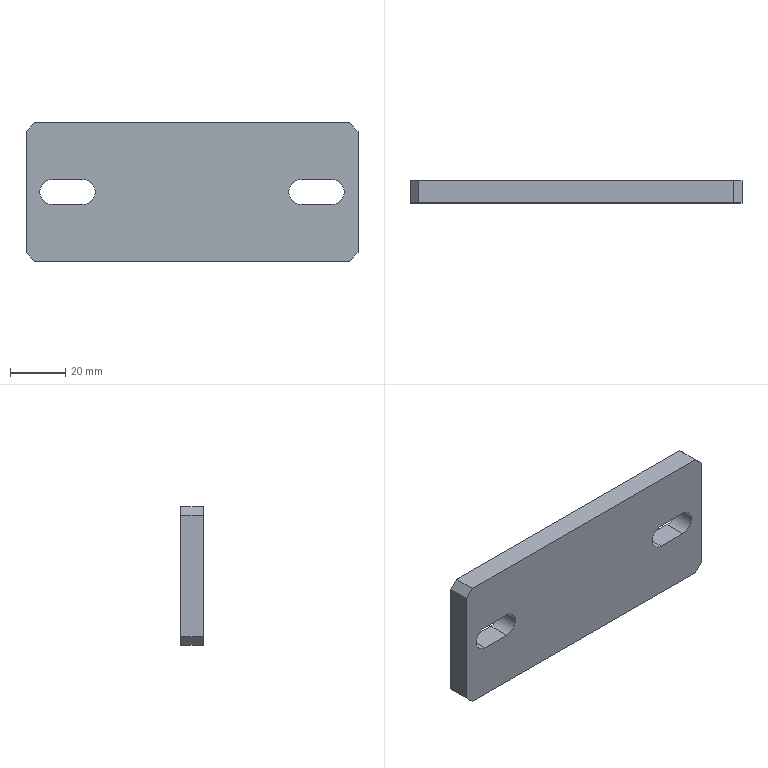Part | STEP file | PN_0013 304 stair handrail mounting plate 120X50X8_Default<As Machined> | 1 solid | 18 faces | box 120 x 8 x 50 mm | volume 45254 mm3 | plane 14 | cylinder 4 | commonest cylinder face diameters 9 x4
STEP:
#1=CARTESIAN_POINT('',(0.,0.,0.));
#2=DIRECTION('',(0.,0.,1.));
#3=DIRECTION('',(1.,0.,0.));
#4=AXIS2_PLACEMENT_3D('',#1,#2,#3);
#5=CARTESIAN_POINT('',(-50.5,0.,4.5));
#6=VERTEX_POINT('',#5);
#7=CARTESIAN_POINT('',(-39.5,0.,4.5));
#8=VERTEX_POINT('',#7);
#9=CARTESIAN_POINT('',(-50.5,0.,4.5));
#10=DIRECTION('',(1.,0.,0.));
#11=VECTOR('',#10,1.);
#12=LINE('',#9,#11);
#13=CARTESIAN_POINT('',(0.,0.,0.));
#14=DIRECTION('',(0.,-1.,0.));
#15=DIRECTION('',(0.,0.,-1.));
#16=AXIS2_PLACEMENT_3D('',#13,#14,#15);
#17=PLANE('',#16);
#18=CARTESIAN_POINT('',(-4.5,-50.5));
#19=DIRECTION('',(0.,1.));
#20=VECTOR('',#19,1.);
#21=LINE('',#18,#20);
#22=(GEOMETRIC_REPRESENTATION_CONTEXT(2)PARAMETRIC_REPRESENTATION_CONTEXT()REPRESENTATION_CONTEXT('',''));
#23=DEFINITIONAL_REPRESENTATION('',(#21),#22);
#24=PCURVE('',#17,#23);
#25=CARTESIAN_POINT('',(-50.5,8.,4.5));
#26=DIRECTION('',(0.,0.,1.));
#27=DIRECTION('',(1.,0.,0.));
#28=AXIS2_PLACEMENT_3D('',#25,#26,#27);
#29=PLANE('',#28);
#30=CARTESIAN_POINT('',(0.,-8.));
#31=DIRECTION('',(1.,0.));
#32=VECTOR('',#31,1.);
#33=LINE('',#30,#32);
#34=(GEOMETRIC_REPRESENTATION_CONTEXT(2)PARAMETRIC_REPRESENTATION_CONTEXT()REPRESENTATION_CONTEXT('',''));
#35=DEFINITIONAL_REPRESENTATION('',(#33),#34);
#36=PCURVE('',#29,#35);
#37=SURFACE_CURVE('',#12,(#24,#36),.PCURVE_S1.);
#38=EDGE_CURVE('',#6,#8,#37,.T.);
#39=ORIENTED_EDGE('',*,*,#38,.T.);
#40=CARTESIAN_POINT('',(-39.5,0.,-4.5));
#41=VERTEX_POINT('',#40);
#42=CARTESIAN_POINT('',(-39.5,0.,0.));
#43=DIRECTION('',(0.,1.,0.));
#44=DIRECTION('',(0.,0.,1.));
#45=AXIS2_PLACEMENT_3D('',#42,#43,#44);
#46=CIRCLE('',#45,4.5);
#47=CARTESIAN_POINT('',(-4.5,-39.5));
#48=CARTESIAN_POINT('',(-4.5,-31.706));
#49=CARTESIAN_POINT('',(2.25,-35.603));
#50=CARTESIAN_POINT('',(9.,-39.5));
#51=CARTESIAN_POINT('',(2.25,-43.397));
#52=CARTESIAN_POINT('',(-4.5,-47.294));
#53=CARTESIAN_POINT('',(-4.5,-39.5));
#54=(BOUNDED_CURVE()B_SPLINE_CURVE(2,(#47,#48,#49,#50,#51,#52,#53),.UNSPECIFIED.,.T.,.F.)B_SPLINE_CURVE_WITH_KNOTS((1,2,2,2,2,1),(-2.094,0.,2.094,4.189,6.283,8.378),.UNSPECIFIED.)CURVE()GEOMETRIC_REPRESENTATION_ITEM()RATIONAL_B_SPLINE_CURVE((1.,0.5,1.,0.5,1.,0.5,1.))REPRESENTATION_ITEM(''));
#55=(GEOMETRIC_REPRESENTATION_CONTEXT(2)PARAMETRIC_REPRESENTATION_CONTEXT()REPRESENTATION_CONTEXT('',''));
#56=DEFINITIONAL_REPRESENTATION('',(#54),#55);
#57=PCURVE('',#17,#56);
#58=CARTESIAN_POINT('',(-39.5,8.,0.));
#59=DIRECTION('',(0.,1.,0.));
#60=DIRECTION('',(0.,0.,1.));
#61=AXIS2_PLACEMENT_3D('',#58,#59,#60);
#62=CYLINDRICAL_SURFACE('',#61,4.5);
#63=CARTESIAN_POINT('',(0.,-8.));
#64=DIRECTION('',(1.,0.));
#65=VECTOR('',#64,1.);
#66=LINE('',#63,#65);
#67=(GEOMETRIC_REPRESENTATION_CONTEXT(2)PARAMETRIC_REPRESENTATION_CONTEXT()REPRESENTATION_CONTEXT('',''));
#68=DEFINITIONAL_REPRESENTATION('',(#66),#67);
#69=PCURVE('',#62,#68);
#70=SURFACE_CURVE('',#46,(#57,#69),.PCURVE_S1.);
#71=EDGE_CURVE('',#8,#41,#70,.T.);
#72=ORIENTED_EDGE('',*,*,#71,.T.);
#73=CARTESIAN_POINT('',(-50.5,0.,-4.5));
#74=VERTEX_POINT('',#73);
#75=CARTESIAN_POINT('',(-50.5,0.,-4.5));
#76=DIRECTION('',(1.,0.,0.));
#77=VECTOR('',#76,1.);
#78=LINE('',#75,#77);
#79=CARTESIAN_POINT('',(4.5,-50.5));
#80=DIRECTION('',(0.,1.));
#81=VECTOR('',#80,1.);
#82=LINE('',#79,#81);
#83=(GEOMETRIC_REPRESENTATION_CONTEXT(2)PARAMETRIC_REPRESENTATION_CONTEXT()REPRESENTATION_CONTEXT('',''));
#84=DEFINITIONAL_REPRESENTATION('',(#82),#83);
#85=PCURVE('',#17,#84);
#86=CARTESIAN_POINT('',(-50.5,8.,-4.5));
#87=DIRECTION('',(0.,0.,-1.));
#88=DIRECTION('',(-1.,0.,0.));
#89=AXIS2_PLACEMENT_3D('',#86,#87,#88);
#90=PLANE('',#89);
#91=CARTESIAN_POINT('',(0.,-8.));
#92=DIRECTION('',(-1.,0.));
#93=VECTOR('',#92,1.);
#94=LINE('',#91,#93);
#95=(GEOMETRIC_REPRESENTATION_CONTEXT(2)PARAMETRIC_REPRESENTATION_CONTEXT()REPRESENTATION_CONTEXT('',''));
#96=DEFINITIONAL_REPRESENTATION('',(#94),#95);
#97=PCURVE('',#90,#96);
#98=SURFACE_CURVE('',#78,(#85,#97),.PCURVE_S1.);
#99=EDGE_CURVE('',#74,#41,#98,.T.);
#100=ORIENTED_EDGE('',*,*,#99,.F.);
#101=CARTESIAN_POINT('',(-50.5,0.,0.));
#102=DIRECTION('',(0.,1.,0.));
#103=DIRECTION('',(0.,0.,1.));
#104=AXIS2_PLACEMENT_3D('',#101,#102,#103);
#105=CIRCLE('',#104,4.5);
#106=CARTESIAN_POINT('',(-4.5,-50.5));
#107=CARTESIAN_POINT('',(-4.5,-42.706));
#108=CARTESIAN_POINT('',(2.25,-46.603));
#109=CARTESIAN_POINT('',(9.,-50.5));
#110=CARTESIAN_POINT('',(2.25,-54.397));
#111=CARTESIAN_POINT('',(-4.5,-58.294));
#112=CARTESIAN_POINT('',(-4.5,-50.5));
#113=(BOUNDED_CURVE()B_SPLINE_CURVE(2,(#106,#107,#108,#109,#110,#111,#112),.UNSPECIFIED.,.T.,.F.)B_SPLINE_CURVE_WITH_KNOTS((1,2,2,2,2,1),(-2.094,0.,2.094,4.189,6.283,8.378),.UNSPECIFIED.)CURVE()GEOMETRIC_REPRESENTATION_ITEM()RATIONAL_B_SPLINE_CURVE((1.,0.5,1.,0.5,1.,0.5,1.))REPRESENTATION_ITEM(''));
#114=(GEOMETRIC_REPRESENTATION_CONTEXT(2)PARAMETRIC_REPRESENTATION_CONTEXT()REPRESENTATION_CONTEXT('',''));
#115=DEFINITIONAL_REPRESENTATION('',(#113),#114);
#116=PCURVE('',#17,#115);
#117=CARTESIAN_POINT('',(-50.5,8.,0.));
#118=DIRECTION('',(0.,1.,0.));
#119=DIRECTION('',(0.,0.,1.));
#120=AXIS2_PLACEMENT_3D('',#117,#118,#119);
#121=CYLINDRICAL_SURFACE('',#120,4.5);
#122=CARTESIAN_POINT('',(0.,-8.));
#123=DIRECTION('',(1.,0.));
#124=VECTOR('',#123,1.);
#125=LINE('',#122,#124);
#126=(GEOMETRIC_REPRESENTATION_CONTEXT(2)PARAMETRIC_REPRESENTATION_CONTEXT()REPRESENTATION_CONTEXT('',''));
#127=DEFINITIONAL_REPRESENTATION('',(#125),#126);
#128=PCURVE('',#121,#127);
#129=SURFACE_CURVE('',#105,(#116,#128),.PCURVE_S1.);
#130=EDGE_CURVE('',#74,#6,#129,.T.);
#131=ORIENTED_EDGE('',*,*,#130,.T.);
#132=EDGE_LOOP('',(#39,#72,#100,#131));
#133=FACE_BOUND('',#132,.T.);
#134=CARTESIAN_POINT('',(57.,0.,-25.));
#135=VERTEX_POINT('',#134);
#136=CARTESIAN_POINT('',(-57.,0.,-25.));
#137=VERTEX_POINT('',#136);
#138=CARTESIAN_POINT('',(-60.,0.,-25.));
#139=DIRECTION('',(-1.,0.,0.));
#140=VECTOR('',#139,1.);
#141=LINE('',#138,#140);
#142=CARTESIAN_POINT('',(25.,-60.));
#143=DIRECTION('',(0.,-1.));
#144=VECTOR('',#143,1.);
#145=LINE('',#142,#144);
#146=(GEOMETRIC_REPRESENTATION_CONTEXT(2)PARAMETRIC_REPRESENTATION_CONTEXT()REPRESENTATION_CONTEXT('',''));
#147=DEFINITIONAL_REPRESENTATION('',(#145),#146);
#148=PCURVE('',#17,#147);
#149=CARTESIAN_POINT('',(-60.,8.,-25.));
#150=DIRECTION('',(0.,0.,1.));
#151=DIRECTION('',(1.,0.,0.));
#152=AXIS2_PLACEMENT_3D('',#149,#150,#151);
#153=PLANE('',#152);
#154=CARTESIAN_POINT('',(0.,-8.));
#155=DIRECTION('',(-1.,0.));
#156=VECTOR('',#155,1.);
#157=LINE('',#154,#156);
#158=(GEOMETRIC_REPRESENTATION_CONTEXT(2)PARAMETRIC_REPRESENTATION_CONTEXT()REPRESENTATION_CONTEXT('',''));
#159=DEFINITIONAL_REPRESENTATION('',(#157),#158);
#160=PCURVE('',#153,#159);
#161=SURFACE_CURVE('',#141,(#148,#160),.PCURVE_S1.);
#162=EDGE_CURVE('',#135,#137,#161,.T.);
#163=ORIENTED_EDGE('',*,*,#162,.F.);
#164=CARTESIAN_POINT('',(60.,0.,-22.));
#165=VERTEX_POINT('',#164);
#166=CARTESIAN_POINT('',(41.,0.,-41.));
#167=DIRECTION('',(0.7071,0.,0.7071));
#168=VECTOR('',#167,1.);
#169=LINE('',#166,#168);
#170=CARTESIAN_POINT('',(41.,41.));
#171=DIRECTION('',(-0.7071,0.7071));
#172=VECTOR('',#171,1.);
#173=LINE('',#170,#172);
#174=(GEOMETRIC_REPRESENTATION_CONTEXT(2)PARAMETRIC_REPRESENTATION_CONTEXT()REPRESENTATION_CONTEXT('',''));
#175=DEFINITIONAL_REPRESENTATION('',(#173),#174);
#176=PCURVE('',#17,#175);
#177=CARTESIAN_POINT('',(57.,8.,-25.));
#178=DIRECTION('',(-0.7071,0.,0.7071));
#179=DIRECTION('',(0.,-1.,0.));
#180=AXIS2_PLACEMENT_3D('',#177,#178,#179);
#181=PLANE('',#180);
#182=CARTESIAN_POINT('',(8.,-22.627));
#183=DIRECTION('',(0.,1.));
#184=VECTOR('',#183,1.);
#185=LINE('',#182,#184);
#186=(GEOMETRIC_REPRESENTATION_CONTEXT(2)PARAMETRIC_REPRESENTATION_CONTEXT()REPRESENTATION_CONTEXT('',''));
#187=DEFINITIONAL_REPRESENTATION('',(#185),#186);
#188=PCURVE('',#181,#187);
#189=SURFACE_CURVE('',#169,(#176,#188),.PCURVE_S1.);
#190=EDGE_CURVE('',#135,#165,#189,.T.);
#191=ORIENTED_EDGE('',*,*,#190,.T.);
#192=CARTESIAN_POINT('',(60.,0.,22.));
#193=VERTEX_POINT('',#192);
#194=CARTESIAN_POINT('',(60.,0.,25.));
#195=DIRECTION('',(0.,0.,-1.));
#196=VECTOR('',#195,1.);
#197=LINE('',#194,#196);
#198=CARTESIAN_POINT('',(-25.,60.));
#199=DIRECTION('',(1.,0.));
#200=VECTOR('',#199,1.);
#201=LINE('',#198,#200);
#202=(GEOMETRIC_REPRESENTATION_CONTEXT(2)PARAMETRIC_REPRESENTATION_CONTEXT()REPRESENTATION_CONTEXT('',''));
#203=DEFINITIONAL_REPRESENTATION('',(#201),#202);
#204=PCURVE('',#17,#203);
#205=CARTESIAN_POINT('',(60.,8.,25.));
#206=DIRECTION('',(-1.,0.,0.));
#207=DIRECTION('',(0.,0.,1.));
#208=AXIS2_PLACEMENT_3D('',#205,#206,#207);
#209=PLANE('',#208);
#210=CARTESIAN_POINT('',(0.,-8.));
#211=DIRECTION('',(-1.,0.));
#212=VECTOR('',#211,1.);
#213=LINE('',#210,#212);
#214=(GEOMETRIC_REPRESENTATION_CONTEXT(2)PARAMETRIC_REPRESENTATION_CONTEXT()REPRESENTATION_CONTEXT('',''));
#215=DEFINITIONAL_REPRESENTATION('',(#213),#214);
#216=PCURVE('',#209,#215);
#217=SURFACE_CURVE('',#197,(#204,#216),.PCURVE_S1.);
#218=EDGE_CURVE('',#193,#165,#217,.T.);
#219=ORIENTED_EDGE('',*,*,#218,.F.);
#220=CARTESIAN_POINT('',(57.,0.,25.));
#221=VERTEX_POINT('',#220);
#222=CARTESIAN_POINT('',(41.,0.,41.));
#223=DIRECTION('',(-0.7071,0.,0.7071));
#224=VECTOR('',#223,1.);
#225=LINE('',#222,#224);
#226=CARTESIAN_POINT('',(-41.,41.));
#227=DIRECTION('',(-0.7071,-0.7071));
#228=VECTOR('',#227,1.);
#229=LINE('',#226,#228);
#230=(GEOMETRIC_REPRESENTATION_CONTEXT(2)PARAMETRIC_REPRESENTATION_CONTEXT()REPRESENTATION_CONTEXT('',''));
#231=DEFINITIONAL_REPRESENTATION('',(#229),#230);
#232=PCURVE('',#17,#231);
#233=CARTESIAN_POINT('',(60.,8.,22.));
#234=DIRECTION('',(-0.7071,0.,-0.7071));
#235=DIRECTION('',(0.,-1.,0.));
#236=AXIS2_PLACEMENT_3D('',#233,#234,#235);
#237=PLANE('',#236);
#238=CARTESIAN_POINT('',(8.,26.87));
#239=DIRECTION('',(0.,1.));
#240=VECTOR('',#239,1.);
#241=LINE('',#238,#240);
#242=(GEOMETRIC_REPRESENTATION_CONTEXT(2)PARAMETRIC_REPRESENTATION_CONTEXT()REPRESENTATION_CONTEXT('',''));
#243=DEFINITIONAL_REPRESENTATION('',(#241),#242);
#244=PCURVE('',#237,#243);
#245=SURFACE_CURVE('',#225,(#232,#244),.PCURVE_S1.);
#246=EDGE_CURVE('',#193,#221,#245,.T.);
#247=ORIENTED_EDGE('',*,*,#246,.T.);
#248=CARTESIAN_POINT('',(-57.,0.,25.));
#249=VERTEX_POINT('',#248);
#250=CARTESIAN_POINT('',(-60.,0.,25.));
#251=DIRECTION('',(1.,0.,0.));
#252=VECTOR('',#251,1.);
#253=LINE('',#250,#252);
#254=CARTESIAN_POINT('',(-25.,-60.));
#255=DIRECTION('',(0.,1.));
#256=VECTOR('',#255,1.);
#257=LINE('',#254,#256);
#258=(GEOMETRIC_REPRESENTATION_CONTEXT(2)PARAMETRIC_REPRESENTATION_CONTEXT()REPRESENTATION_CONTEXT('',''));
#259=DEFINITIONAL_REPRESENTATION('',(#257),#258);
#260=PCURVE('',#17,#259);
#261=CARTESIAN_POINT('',(-60.,8.,25.));
#262=DIRECTION('',(0.,0.,-1.));
#263=DIRECTION('',(-1.,0.,0.));
#264=AXIS2_PLACEMENT_3D('',#261,#262,#263);
#265=PLANE('',#264);
#266=CARTESIAN_POINT('',(0.,-8.));
#267=DIRECTION('',(-1.,0.));
#268=VECTOR('',#267,1.);
#269=LINE('',#266,#268);
#270=(GEOMETRIC_REPRESENTATION_CONTEXT(2)PARAMETRIC_REPRESENTATION_CONTEXT()REPRESENTATION_CONTEXT('',''));
#271=DEFINITIONAL_REPRESENTATION('',(#269),#270);
#272=PCURVE('',#265,#271);
#273=SURFACE_CURVE('',#253,(#260,#272),.PCURVE_S1.);
#274=EDGE_CURVE('',#249,#221,#273,.T.);
#275=ORIENTED_EDGE('',*,*,#274,.F.);
#276=CARTESIAN_POINT('',(-60.,0.,22.));
#277=VERTEX_POINT('',#276);
#278=CARTESIAN_POINT('',(-41.,0.,41.));
#279=DIRECTION('',(-0.7071,0.,-0.7071));
#280=VECTOR('',#279,1.);
#281=LINE('',#278,#280);
#282=CARTESIAN_POINT('',(-41.,-41.));
#283=DIRECTION('',(0.7071,-0.7071));
#284=VECTOR('',#283,1.);
#285=LINE('',#282,#284);
#286=(GEOMETRIC_REPRESENTATION_CONTEXT(2)PARAMETRIC_REPRESENTATION_CONTEXT()REPRESENTATION_CONTEXT('',''));
#287=DEFINITIONAL_REPRESENTATION('',(#285),#286);
#288=PCURVE('',#17,#287);
#289=CARTESIAN_POINT('',(-57.,8.,25.));
#290=DIRECTION('',(0.7071,0.,-0.7071));
#291=DIRECTION('',(0.,-1.,0.));
#292=AXIS2_PLACEMENT_3D('',#289,#290,#291);
#293=PLANE('',#292);
#294=CARTESIAN_POINT('',(8.,-22.627));
#295=DIRECTION('',(0.,1.));
#296=VECTOR('',#295,1.);
#297=LINE('',#294,#296);
#298=(GEOMETRIC_REPRESENTATION_CONTEXT(2)PARAMETRIC_REPRESENTATION_CONTEXT()REPRESENTATION_CONTEXT('',''));
#299=DEFINITIONAL_REPRESENTATION('',(#297),#298);
#300=PCURVE('',#293,#299);
#301=SURFACE_CURVE('',#281,(#288,#300),.PCURVE_S1.);
#302=EDGE_CURVE('',#249,#277,#301,.T.);
#303=ORIENTED_EDGE('',*,*,#302,.T.);
#304=CARTESIAN_POINT('',(-60.,0.,-22.));
#305=VERTEX_POINT('',#304);
#306=CARTESIAN_POINT('',(-60.,0.,25.));
#307=DIRECTION('',(0.,0.,1.));
#308=VECTOR('',#307,1.);
#309=LINE('',#306,#308);
#310=CARTESIAN_POINT('',(-25.,-60.));
#311=DIRECTION('',(-1.,0.));
#312=VECTOR('',#311,1.);
#313=LINE('',#310,#312);
#314=(GEOMETRIC_REPRESENTATION_CONTEXT(2)PARAMETRIC_REPRESENTATION_CONTEXT()REPRESENTATION_CONTEXT('',''));
#315=DEFINITIONAL_REPRESENTATION('',(#313),#314);
#316=PCURVE('',#17,#315);
#317=CARTESIAN_POINT('',(-60.,8.,25.));
#318=DIRECTION('',(1.,0.,0.));
#319=DIRECTION('',(0.,0.,-1.));
#320=AXIS2_PLACEMENT_3D('',#317,#318,#319);
#321=PLANE('',#320);
#322=CARTESIAN_POINT('',(0.,-8.));
#323=DIRECTION('',(-1.,0.));
#324=VECTOR('',#323,1.);
#325=LINE('',#322,#324);
#326=(GEOMETRIC_REPRESENTATION_CONTEXT(2)PARAMETRIC_REPRESENTATION_CONTEXT()REPRESENTATION_CONTEXT('',''));
#327=DEFINITIONAL_REPRESENTATION('',(#325),#326);
#328=PCURVE('',#321,#327);
#329=SURFACE_CURVE('',#309,(#316,#328),.PCURVE_S1.);
#330=EDGE_CURVE('',#305,#277,#329,.T.);
#331=ORIENTED_EDGE('',*,*,#330,.F.);
#332=CARTESIAN_POINT('',(-41.,0.,-41.));
#333=DIRECTION('',(0.7071,0.,-0.7071));
#334=VECTOR('',#333,1.);
#335=LINE('',#332,#334);
#336=CARTESIAN_POINT('',(41.,-41.));
#337=DIRECTION('',(0.7071,0.7071));
#338=VECTOR('',#337,1.);
#339=LINE('',#336,#338);
#340=(GEOMETRIC_REPRESENTATION_CONTEXT(2)PARAMETRIC_REPRESENTATION_CONTEXT()REPRESENTATION_CONTEXT('',''));
#341=DEFINITIONAL_REPRESENTATION('',(#339),#340);
#342=PCURVE('',#17,#341);
#343=CARTESIAN_POINT('',(-60.,8.,-22.));
#344=DIRECTION('',(0.7071,0.,0.7071));
#345=DIRECTION('',(0.,-1.,0.));
#346=AXIS2_PLACEMENT_3D('',#343,#344,#345);
#347=PLANE('',#346);
#348=CARTESIAN_POINT('',(8.,26.87));
#349=DIRECTION('',(0.,1.));
#350=VECTOR('',#349,1.);
#351=LINE('',#348,#350);
#352=(GEOMETRIC_REPRESENTATION_CONTEXT(2)PARAMETRIC_REPRESENTATION_CONTEXT()REPRESENTATION_CONTEXT('',''));
#353=DEFINITIONAL_REPRESENTATION('',(#351),#352);
#354=PCURVE('',#347,#353);
#355=SURFACE_CURVE('',#335,(#342,#354),.PCURVE_S1.);
#356=EDGE_CURVE('',#305,#137,#355,.T.);
#357=ORIENTED_EDGE('',*,*,#356,.T.);
#358=EDGE_LOOP('',(#163,#191,#219,#247,#275,#303,#331,#357));
#359=FACE_BOUND('',#358,.T.);
#360=CARTESIAN_POINT('',(39.5,0.,-4.5));
#361=VERTEX_POINT('',#360);
#362=CARTESIAN_POINT('',(39.5,0.,4.5));
#363=VERTEX_POINT('',#362);
#364=CARTESIAN_POINT('',(39.5,0.,0.));
#365=DIRECTION('',(0.,1.,0.));
#366=DIRECTION('',(0.,0.,1.));
#367=AXIS2_PLACEMENT_3D('',#364,#365,#366);
#368=CIRCLE('',#367,4.5);
#369=CARTESIAN_POINT('',(-4.5,39.5));
#370=CARTESIAN_POINT('',(-4.5,47.294));
#371=CARTESIAN_POINT('',(2.25,43.397));
#372=CARTESIAN_POINT('',(9.,39.5));
#373=CARTESIAN_POINT('',(2.25,35.603));
#374=CARTESIAN_POINT('',(-4.5,31.706));
#375=CARTESIAN_POINT('',(-4.5,39.5));
#376=(BOUNDED_CURVE()B_SPLINE_CURVE(2,(#369,#370,#371,#372,#373,#374,#375),.UNSPECIFIED.,.T.,.F.)B_SPLINE_CURVE_WITH_KNOTS((1,2,2,2,2,1),(-2.094,0.,2.094,4.189,6.283,8.378),.UNSPECIFIED.)CURVE()GEOMETRIC_REPRESENTATION_ITEM()RATIONAL_B_SPLINE_CURVE((1.,0.5,1.,0.5,1.,0.5,1.))REPRESENTATION_ITEM(''));
#377=(GEOMETRIC_REPRESENTATION_CONTEXT(2)PARAMETRIC_REPRESENTATION_CONTEXT()REPRESENTATION_CONTEXT('',''));
#378=DEFINITIONAL_REPRESENTATION('',(#376),#377);
#379=PCURVE('',#17,#378);
#380=CARTESIAN_POINT('',(39.5,8.,0.));
#381=DIRECTION('',(0.,1.,0.));
#382=DIRECTION('',(0.,0.,1.));
#383=AXIS2_PLACEMENT_3D('',#380,#381,#382);
#384=CYLINDRICAL_SURFACE('',#383,4.5);
#385=CARTESIAN_POINT('',(0.,-8.));
#386=DIRECTION('',(1.,0.));
#387=VECTOR('',#386,1.);
#388=LINE('',#385,#387);
#389=(GEOMETRIC_REPRESENTATION_CONTEXT(2)PARAMETRIC_REPRESENTATION_CONTEXT()REPRESENTATION_CONTEXT('',''));
#390=DEFINITIONAL_REPRESENTATION('',(#388),#389);
#391=PCURVE('',#384,#390);
#392=SURFACE_CURVE('',#368,(#379,#391),.PCURVE_S1.);
#393=EDGE_CURVE('',#361,#363,#392,.T.);
#394=ORIENTED_EDGE('',*,*,#393,.T.);
#395=CARTESIAN_POINT('',(50.5,0.,4.5));
#396=VERTEX_POINT('',#395);
#397=CARTESIAN_POINT('',(39.5,0.,4.5));
#398=DIRECTION('',(1.,0.,0.));
#399=VECTOR('',#398,1.);
#400=LINE('',#397,#399);
#401=CARTESIAN_POINT('',(-4.5,39.5));
#402=DIRECTION('',(0.,1.));
#403=VECTOR('',#402,1.);
#404=LINE('',#401,#403);
#405=(GEOMETRIC_REPRESENTATION_CONTEXT(2)PARAMETRIC_REPRESENTATION_CONTEXT()REPRESENTATION_CONTEXT('',''));
#406=DEFINITIONAL_REPRESENTATION('',(#404),#405);
#407=PCURVE('',#17,#406);
#408=CARTESIAN_POINT('',(39.5,8.,4.5));
#409=DIRECTION('',(0.,0.,1.));
#410=DIRECTION('',(1.,0.,0.));
#411=AXIS2_PLACEMENT_3D('',#408,#409,#410);
#412=PLANE('',#411);
#413=CARTESIAN_POINT('',(0.,-8.));
#414=DIRECTION('',(1.,0.));
#415=VECTOR('',#414,1.);
#416=LINE('',#413,#415);
#417=(GEOMETRIC_REPRESENTATION_CONTEXT(2)PARAMETRIC_REPRESENTATION_CONTEXT()REPRESENTATION_CONTEXT('',''));
#418=DEFINITIONAL_REPRESENTATION('',(#416),#417);
#419=PCURVE('',#412,#418);
#420=SURFACE_CURVE('',#400,(#407,#419),.PCURVE_S1.);
#421=EDGE_CURVE('',#363,#396,#420,.T.);
#422=ORIENTED_EDGE('',*,*,#421,.T.);
#423=CARTESIAN_POINT('',(50.5,0.,-4.5));
#424=VERTEX_POINT('',#423);
#425=CARTESIAN_POINT('',(50.5,0.,0.));
#426=DIRECTION('',(0.,1.,0.));
#427=DIRECTION('',(0.,0.,1.));
#428=AXIS2_PLACEMENT_3D('',#425,#426,#427);
#429=CIRCLE('',#428,4.5);
#430=CARTESIAN_POINT('',(-4.5,50.5));
#431=CARTESIAN_POINT('',(-4.5,58.294));
#432=CARTESIAN_POINT('',(2.25,54.397));
#433=CARTESIAN_POINT('',(9.,50.5));
#434=CARTESIAN_POINT('',(2.25,46.603));
#435=CARTESIAN_POINT('',(-4.5,42.706));
#436=CARTESIAN_POINT('',(-4.5,50.5));
#437=(BOUNDED_CURVE()B_SPLINE_CURVE(2,(#430,#431,#432,#433,#434,#435,#436),.UNSPECIFIED.,.T.,.F.)B_SPLINE_CURVE_WITH_KNOTS((1,2,2,2,2,1),(-2.094,0.,2.094,4.189,6.283,8.378),.UNSPECIFIED.)CURVE()GEOMETRIC_REPRESENTATION_ITEM()RATIONAL_B_SPLINE_CURVE((1.,0.5,1.,0.5,1.,0.5,1.))REPRESENTATION_ITEM(''));
#438=(GEOMETRIC_REPRESENTATION_CONTEXT(2)PARAMETRIC_REPRESENTATION_CONTEXT()REPRESENTATION_CONTEXT('',''));
#439=DEFINITIONAL_REPRESENTATION('',(#437),#438);
#440=PCURVE('',#17,#439);
#441=CARTESIAN_POINT('',(50.5,8.,0.));
#442=DIRECTION('',(0.,1.,0.));
#443=DIRECTION('',(0.,0.,1.));
#444=AXIS2_PLACEMENT_3D('',#441,#442,#443);
#445=CYLINDRICAL_SURFACE('',#444,4.5);
#446=CARTESIAN_POINT('',(0.,-8.));
#447=DIRECTION('',(1.,0.));
#448=VECTOR('',#447,1.);
#449=LINE('',#446,#448);
#450=(GEOMETRIC_REPRESENTATION_CONTEXT(2)PARAMETRIC_REPRESENTATION_CONTEXT()REPRESENTATION_CONTEXT('',''));
#451=DEFINITIONAL_REPRESENTATION('',(#449),#450);
#452=PCURVE('',#445,#451);
#453=SURFACE_CURVE('',#429,(#440,#452),.PCURVE_S1.);
#454=EDGE_CURVE('',#396,#424,#453,.T.);
#455=ORIENTED_EDGE('',*,*,#454,.T.);
#456=CARTESIAN_POINT('',(39.5,0.,-4.5));
#457=DIRECTION('',(1.,0.,0.));
#458=VECTOR('',#457,1.);
#459=LINE('',#456,#458);
#460=CARTESIAN_POINT('',(4.5,39.5));
#461=DIRECTION('',(0.,1.));
#462=VECTOR('',#461,1.);
#463=LINE('',#460,#462);
#464=(GEOMETRIC_REPRESENTATION_CONTEXT(2)PARAMETRIC_REPRESENTATION_CONTEXT()REPRESENTATION_CONTEXT('',''));
#465=DEFINITIONAL_REPRESENTATION('',(#463),#464);
#466=PCURVE('',#17,#465);
#467=CARTESIAN_POINT('',(39.5,8.,-4.5));
#468=DIRECTION('',(0.,0.,-1.));
#469=DIRECTION('',(-1.,0.,0.));
#470=AXIS2_PLACEMENT_3D('',#467,#468,#469);
#471=PLANE('',#470);
#472=CARTESIAN_POINT('',(0.,-8.));
#473=DIRECTION('',(-1.,0.));
#474=VECTOR('',#473,1.);
#475=LINE('',#472,#474);
#476=(GEOMETRIC_REPRESENTATION_CONTEXT(2)PARAMETRIC_REPRESENTATION_CONTEXT()REPRESENTATION_CONTEXT('',''));
#477=DEFINITIONAL_REPRESENTATION('',(#475),#476);
#478=PCURVE('',#471,#477);
#479=SURFACE_CURVE('',#459,(#466,#478),.PCURVE_S1.);
#480=EDGE_CURVE('',#361,#424,#479,.T.);
#481=ORIENTED_EDGE('',*,*,#480,.F.);
#482=EDGE_LOOP('',(#394,#422,#455,#481));
#483=FACE_BOUND('',#482,.T.);
#484=ADVANCED_FACE('',(#133,#359,#483),#17,.T.);
#485=ORIENTED_EDGE('',*,*,#218,.T.);
#486=CARTESIAN_POINT('',(60.,8.,-22.));
#487=VERTEX_POINT('',#486);
#488=CARTESIAN_POINT('',(60.,8.,-22.));
#489=DIRECTION('',(0.,1.,0.));
#490=VECTOR('',#489,1.);
#491=LINE('',#488,#490);
#492=CARTESIAN_POINT('',(-47.,0.));
#493=DIRECTION('',(0.,1.));
#494=VECTOR('',#493,1.);
#495=LINE('',#492,#494);
#496=(GEOMETRIC_REPRESENTATION_CONTEXT(2)PARAMETRIC_REPRESENTATION_CONTEXT()REPRESENTATION_CONTEXT('',''));
#497=DEFINITIONAL_REPRESENTATION('',(#495),#496);
#498=PCURVE('',#209,#497);
#499=CARTESIAN_POINT('',(0.,4.243));
#500=DIRECTION('',(-1.,0.));
#501=VECTOR('',#500,1.);
#502=LINE('',#499,#501);
#503=(GEOMETRIC_REPRESENTATION_CONTEXT(2)PARAMETRIC_REPRESENTATION_CONTEXT()REPRESENTATION_CONTEXT('',''));
#504=DEFINITIONAL_REPRESENTATION('',(#502),#503);
#505=PCURVE('',#181,#504);
#506=SURFACE_CURVE('',#491,(#498,#505),.PCURVE_S1.);
#507=EDGE_CURVE('',#165,#487,#506,.T.);
#508=ORIENTED_EDGE('',*,*,#507,.T.);
#509=CARTESIAN_POINT('',(60.,8.,22.));
#510=VERTEX_POINT('',#509);
#511=CARTESIAN_POINT('',(60.,8.,25.));
#512=DIRECTION('',(0.,0.,-1.));
#513=VECTOR('',#512,1.);
#514=LINE('',#511,#513);
#515=CARTESIAN_POINT('',(0.,0.));
#516=DIRECTION('',(-1.,0.));
#517=VECTOR('',#516,1.);
#518=LINE('',#515,#517);
#519=(GEOMETRIC_REPRESENTATION_CONTEXT(2)PARAMETRIC_REPRESENTATION_CONTEXT()REPRESENTATION_CONTEXT('',''));
#520=DEFINITIONAL_REPRESENTATION('',(#518),#519);
#521=PCURVE('',#209,#520);
#522=CARTESIAN_POINT('',(0.,8.,0.));
#523=DIRECTION('',(0.,-1.,0.));
#524=DIRECTION('',(0.,0.,-1.));
#525=AXIS2_PLACEMENT_3D('',#522,#523,#524);
#526=PLANE('',#525);
#527=CARTESIAN_POINT('',(-25.,60.));
#528=DIRECTION('',(1.,0.));
#529=VECTOR('',#528,1.);
#530=LINE('',#527,#529);
#531=(GEOMETRIC_REPRESENTATION_CONTEXT(2)PARAMETRIC_REPRESENTATION_CONTEXT()REPRESENTATION_CONTEXT('',''));
#532=DEFINITIONAL_REPRESENTATION('',(#530),#531);
#533=PCURVE('',#526,#532);
#534=SURFACE_CURVE('',#514,(#521,#533),.PCURVE_S1.);
#535=EDGE_CURVE('',#510,#487,#534,.T.);
#536=ORIENTED_EDGE('',*,*,#535,.F.);
#537=CARTESIAN_POINT('',(60.,8.,22.));
#538=DIRECTION('',(0.,-1.,0.));
#539=VECTOR('',#538,1.);
#540=LINE('',#537,#539);
#541=CARTESIAN_POINT('',(-3.,0.));
#542=DIRECTION('',(0.,-1.));
#543=VECTOR('',#542,1.);
#544=LINE('',#541,#543);
#545=(GEOMETRIC_REPRESENTATION_CONTEXT(2)PARAMETRIC_REPRESENTATION_CONTEXT()REPRESENTATION_CONTEXT('',''));
#546=DEFINITIONAL_REPRESENTATION('',(#544),#545);
#547=PCURVE('',#209,#546);
#548=CARTESIAN_POINT('',(0.,0.));
#549=DIRECTION('',(1.,0.));
#550=VECTOR('',#549,1.);
#551=LINE('',#548,#550);
#552=(GEOMETRIC_REPRESENTATION_CONTEXT(2)PARAMETRIC_REPRESENTATION_CONTEXT()REPRESENTATION_CONTEXT('',''));
#553=DEFINITIONAL_REPRESENTATION('',(#551),#552);
#554=PCURVE('',#237,#553);
#555=SURFACE_CURVE('',#540,(#547,#554),.PCURVE_S1.);
#556=EDGE_CURVE('',#510,#193,#555,.T.);
#557=ORIENTED_EDGE('',*,*,#556,.T.);
#558=EDGE_LOOP('',(#485,#508,#536,#557));
#559=FACE_BOUND('',#558,.T.);
#560=ADVANCED_FACE('',(#559),#209,.F.);
#561=CARTESIAN_POINT('',(57.,8.,-25.));
#562=VERTEX_POINT('',#561);
#563=CARTESIAN_POINT('',(-57.,8.,-25.));
#564=VERTEX_POINT('',#563);
#565=CARTESIAN_POINT('',(-60.,8.,-25.));
#566=DIRECTION('',(-1.,0.,0.));
#567=VECTOR('',#566,1.);
#568=LINE('',#565,#567);
#569=CARTESIAN_POINT('',(0.,0.));
#570=DIRECTION('',(-1.,0.));
#571=VECTOR('',#570,1.);
#572=LINE('',#569,#571);
#573=(GEOMETRIC_REPRESENTATION_CONTEXT(2)PARAMETRIC_REPRESENTATION_CONTEXT()REPRESENTATION_CONTEXT('',''));
#574=DEFINITIONAL_REPRESENTATION('',(#572),#573);
#575=PCURVE('',#153,#574);
#576=CARTESIAN_POINT('',(25.,-60.));
#577=DIRECTION('',(0.,-1.));
#578=VECTOR('',#577,1.);
#579=LINE('',#576,#578);
#580=(GEOMETRIC_REPRESENTATION_CONTEXT(2)PARAMETRIC_REPRESENTATION_CONTEXT()REPRESENTATION_CONTEXT('',''));
#581=DEFINITIONAL_REPRESENTATION('',(#579),#580);
#582=PCURVE('',#526,#581);
#583=SURFACE_CURVE('',#568,(#575,#582),.PCURVE_S1.);
#584=EDGE_CURVE('',#562,#564,#583,.T.);
#585=ORIENTED_EDGE('',*,*,#584,.F.);
#586=CARTESIAN_POINT('',(57.,8.,-25.));
#587=DIRECTION('',(0.,-1.,0.));
#588=VECTOR('',#587,1.);
#589=LINE('',#586,#588);
#590=CARTESIAN_POINT('',(117.,0.));
#591=DIRECTION('',(0.,-1.));
#592=VECTOR('',#591,1.);
#593=LINE('',#590,#592);
#594=(GEOMETRIC_REPRESENTATION_CONTEXT(2)PARAMETRIC_REPRESENTATION_CONTEXT()REPRESENTATION_CONTEXT('',''));
#595=DEFINITIONAL_REPRESENTATION('',(#593),#594);
#596=PCURVE('',#153,#595);
#597=CARTESIAN_POINT('',(0.,0.));
#598=DIRECTION('',(1.,0.));
#599=VECTOR('',#598,1.);
#600=LINE('',#597,#599);
#601=(GEOMETRIC_REPRESENTATION_CONTEXT(2)PARAMETRIC_REPRESENTATION_CONTEXT()REPRESENTATION_CONTEXT('',''));
#602=DEFINITIONAL_REPRESENTATION('',(#600),#601);
#603=PCURVE('',#181,#602);
#604=SURFACE_CURVE('',#589,(#596,#603),.PCURVE_S1.);
#605=EDGE_CURVE('',#562,#135,#604,.T.);
#606=ORIENTED_EDGE('',*,*,#605,.T.);
#607=ORIENTED_EDGE('',*,*,#162,.T.);
#608=CARTESIAN_POINT('',(-57.,8.,-25.));
#609=DIRECTION('',(0.,1.,0.));
#610=VECTOR('',#609,1.);
#611=LINE('',#608,#610);
#612=CARTESIAN_POINT('',(3.,0.));
#613=DIRECTION('',(0.,1.));
#614=VECTOR('',#613,1.);
#615=LINE('',#612,#614);
#616=(GEOMETRIC_REPRESENTATION_CONTEXT(2)PARAMETRIC_REPRESENTATION_CONTEXT()REPRESENTATION_CONTEXT('',''));
#617=DEFINITIONAL_REPRESENTATION('',(#615),#616);
#618=PCURVE('',#153,#617);
#619=CARTESIAN_POINT('',(0.,4.243));
#620=DIRECTION('',(-1.,0.));
#621=VECTOR('',#620,1.);
#622=LINE('',#619,#621);
#623=(GEOMETRIC_REPRESENTATION_CONTEXT(2)PARAMETRIC_REPRESENTATION_CONTEXT()REPRESENTATION_CONTEXT('',''));
#624=DEFINITIONAL_REPRESENTATION('',(#622),#623);
#625=PCURVE('',#347,#624);
#626=SURFACE_CURVE('',#611,(#618,#625),.PCURVE_S1.);
#627=EDGE_CURVE('',#137,#564,#626,.T.);
#628=ORIENTED_EDGE('',*,*,#627,.T.);
#629=EDGE_LOOP('',(#585,#606,#607,#628));
#630=FACE_BOUND('',#629,.T.);
#631=ADVANCED_FACE('',(#630),#153,.F.);
#632=ORIENTED_EDGE('',*,*,#330,.T.);
#633=CARTESIAN_POINT('',(-60.,8.,22.));
#634=VERTEX_POINT('',#633);
#635=CARTESIAN_POINT('',(-60.,8.,22.));
#636=DIRECTION('',(0.,1.,0.));
#637=VECTOR('',#636,1.);
#638=LINE('',#635,#637);
#639=CARTESIAN_POINT('',(3.,0.));
#640=DIRECTION('',(0.,1.));
#641=VECTOR('',#640,1.);
#642=LINE('',#639,#641);
#643=(GEOMETRIC_REPRESENTATION_CONTEXT(2)PARAMETRIC_REPRESENTATION_CONTEXT()REPRESENTATION_CONTEXT('',''));
#644=DEFINITIONAL_REPRESENTATION('',(#642),#643);
#645=PCURVE('',#321,#644);
#646=CARTESIAN_POINT('',(0.,4.243));
#647=DIRECTION('',(-1.,0.));
#648=VECTOR('',#647,1.);
#649=LINE('',#646,#648);
#650=(GEOMETRIC_REPRESENTATION_CONTEXT(2)PARAMETRIC_REPRESENTATION_CONTEXT()REPRESENTATION_CONTEXT('',''));
#651=DEFINITIONAL_REPRESENTATION('',(#649),#650);
#652=PCURVE('',#293,#651);
#653=SURFACE_CURVE('',#638,(#645,#652),.PCURVE_S1.);
#654=EDGE_CURVE('',#277,#634,#653,.T.);
#655=ORIENTED_EDGE('',*,*,#654,.T.);
#656=CARTESIAN_POINT('',(-60.,8.,-22.));
#657=VERTEX_POINT('',#656);
#658=CARTESIAN_POINT('',(-60.,8.,25.));
#659=DIRECTION('',(0.,0.,1.));
#660=VECTOR('',#659,1.);
#661=LINE('',#658,#660);
#662=CARTESIAN_POINT('',(0.,0.));
#663=DIRECTION('',(-1.,0.));
#664=VECTOR('',#663,1.);
#665=LINE('',#662,#664);
#666=(GEOMETRIC_REPRESENTATION_CONTEXT(2)PARAMETRIC_REPRESENTATION_CONTEXT()REPRESENTATION_CONTEXT('',''));
#667=DEFINITIONAL_REPRESENTATION('',(#665),#666);
#668=PCURVE('',#321,#667);
#669=CARTESIAN_POINT('',(-25.,-60.));
#670=DIRECTION('',(-1.,0.));
#671=VECTOR('',#670,1.);
#672=LINE('',#669,#671);
#673=(GEOMETRIC_REPRESENTATION_CONTEXT(2)PARAMETRIC_REPRESENTATION_CONTEXT()REPRESENTATION_CONTEXT('',''));
#674=DEFINITIONAL_REPRESENTATION('',(#672),#673);
#675=PCURVE('',#526,#674);
#676=SURFACE_CURVE('',#661,(#668,#675),.PCURVE_S1.);
#677=EDGE_CURVE('',#657,#634,#676,.T.);
#678=ORIENTED_EDGE('',*,*,#677,.F.);
#679=CARTESIAN_POINT('',(-60.,8.,-22.));
#680=DIRECTION('',(0.,-1.,0.));
#681=VECTOR('',#680,1.);
#682=LINE('',#679,#681);
#683=CARTESIAN_POINT('',(47.,0.));
#684=DIRECTION('',(0.,-1.));
#685=VECTOR('',#684,1.);
#686=LINE('',#683,#685);
#687=(GEOMETRIC_REPRESENTATION_CONTEXT(2)PARAMETRIC_REPRESENTATION_CONTEXT()REPRESENTATION_CONTEXT('',''));
#688=DEFINITIONAL_REPRESENTATION('',(#686),#687);
#689=PCURVE('',#321,#688);
#690=CARTESIAN_POINT('',(0.,0.));
#691=DIRECTION('',(1.,0.));
#692=VECTOR('',#691,1.);
#693=LINE('',#690,#692);
#694=(GEOMETRIC_REPRESENTATION_CONTEXT(2)PARAMETRIC_REPRESENTATION_CONTEXT()REPRESENTATION_CONTEXT('',''));
#695=DEFINITIONAL_REPRESENTATION('',(#693),#694);
#696=PCURVE('',#347,#695);
#697=SURFACE_CURVE('',#682,(#689,#696),.PCURVE_S1.);
#698=EDGE_CURVE('',#657,#305,#697,.T.);
#699=ORIENTED_EDGE('',*,*,#698,.T.);
#700=EDGE_LOOP('',(#632,#655,#678,#699));
#701=FACE_BOUND('',#700,.T.);
#702=ADVANCED_FACE('',(#701),#321,.F.);
#703=ORIENTED_EDGE('',*,*,#274,.T.);
#704=CARTESIAN_POINT('',(57.,8.,25.));
#705=VERTEX_POINT('',#704);
#706=CARTESIAN_POINT('',(57.,8.,25.));
#707=DIRECTION('',(0.,1.,0.));
#708=VECTOR('',#707,1.);
#709=LINE('',#706,#708);
#710=CARTESIAN_POINT('',(-117.,0.));
#711=DIRECTION('',(0.,1.));
#712=VECTOR('',#711,1.);
#713=LINE('',#710,#712);
#714=(GEOMETRIC_REPRESENTATION_CONTEXT(2)PARAMETRIC_REPRESENTATION_CONTEXT()REPRESENTATION_CONTEXT('',''));
#715=DEFINITIONAL_REPRESENTATION('',(#713),#714);
#716=PCURVE('',#265,#715);
#717=CARTESIAN_POINT('',(0.,4.243));
#718=DIRECTION('',(-1.,0.));
#719=VECTOR('',#718,1.);
#720=LINE('',#717,#719);
#721=(GEOMETRIC_REPRESENTATION_CONTEXT(2)PARAMETRIC_REPRESENTATION_CONTEXT()REPRESENTATION_CONTEXT('',''));
#722=DEFINITIONAL_REPRESENTATION('',(#720),#721);
#723=PCURVE('',#237,#722);
#724=SURFACE_CURVE('',#709,(#716,#723),.PCURVE_S1.);
#725=EDGE_CURVE('',#221,#705,#724,.T.);
#726=ORIENTED_EDGE('',*,*,#725,.T.);
#727=CARTESIAN_POINT('',(-57.,8.,25.));
#728=VERTEX_POINT('',#727);
#729=CARTESIAN_POINT('',(-60.,8.,25.));
#730=DIRECTION('',(1.,0.,0.));
#731=VECTOR('',#730,1.);
#732=LINE('',#729,#731);
#733=CARTESIAN_POINT('',(0.,0.));
#734=DIRECTION('',(-1.,0.));
#735=VECTOR('',#734,1.);
#736=LINE('',#733,#735);
#737=(GEOMETRIC_REPRESENTATION_CONTEXT(2)PARAMETRIC_REPRESENTATION_CONTEXT()REPRESENTATION_CONTEXT('',''));
#738=DEFINITIONAL_REPRESENTATION('',(#736),#737);
#739=PCURVE('',#265,#738);
#740=CARTESIAN_POINT('',(-25.,-60.));
#741=DIRECTION('',(0.,1.));
#742=VECTOR('',#741,1.);
#743=LINE('',#740,#742);
#744=(GEOMETRIC_REPRESENTATION_CONTEXT(2)PARAMETRIC_REPRESENTATION_CONTEXT()REPRESENTATION_CONTEXT('',''));
#745=DEFINITIONAL_REPRESENTATION('',(#743),#744);
#746=PCURVE('',#526,#745);
#747=SURFACE_CURVE('',#732,(#739,#746),.PCURVE_S1.);
#748=EDGE_CURVE('',#728,#705,#747,.T.);
#749=ORIENTED_EDGE('',*,*,#748,.F.);
#750=CARTESIAN_POINT('',(-57.,8.,25.));
#751=DIRECTION('',(0.,-1.,0.));
#752=VECTOR('',#751,1.);
#753=LINE('',#750,#752);
#754=CARTESIAN_POINT('',(-3.,0.));
#755=DIRECTION('',(0.,-1.));
#756=VECTOR('',#755,1.);
#757=LINE('',#754,#756);
#758=(GEOMETRIC_REPRESENTATION_CONTEXT(2)PARAMETRIC_REPRESENTATION_CONTEXT()REPRESENTATION_CONTEXT('',''));
#759=DEFINITIONAL_REPRESENTATION('',(#757),#758);
#760=PCURVE('',#265,#759);
#761=CARTESIAN_POINT('',(0.,0.));
#762=DIRECTION('',(1.,0.));
#763=VECTOR('',#762,1.);
#764=LINE('',#761,#763);
#765=(GEOMETRIC_REPRESENTATION_CONTEXT(2)PARAMETRIC_REPRESENTATION_CONTEXT()REPRESENTATION_CONTEXT('',''));
#766=DEFINITIONAL_REPRESENTATION('',(#764),#765);
#767=PCURVE('',#293,#766);
#768=SURFACE_CURVE('',#753,(#760,#767),.PCURVE_S1.);
#769=EDGE_CURVE('',#728,#249,#768,.T.);
#770=ORIENTED_EDGE('',*,*,#769,.T.);
#771=EDGE_LOOP('',(#703,#726,#749,#770));
#772=FACE_BOUND('',#771,.T.);
#773=ADVANCED_FACE('',(#772),#265,.F.);
#774=CARTESIAN_POINT('',(39.5,8.,-4.5));
#775=VERTEX_POINT('',#774);
#776=CARTESIAN_POINT('',(39.5,8.,4.5));
#777=VERTEX_POINT('',#776);
#778=CARTESIAN_POINT('',(39.5,8.,0.));
#779=DIRECTION('',(0.,1.,0.));
#780=DIRECTION('',(0.,0.,1.));
#781=AXIS2_PLACEMENT_3D('',#778,#779,#780);
#782=CIRCLE('',#781,4.5);
#783=CARTESIAN_POINT('',(-4.5,39.5));
#784=CARTESIAN_POINT('',(-4.5,47.294));
#785=CARTESIAN_POINT('',(2.25,43.397));
#786=CARTESIAN_POINT('',(9.,39.5));
#787=CARTESIAN_POINT('',(2.25,35.603));
#788=CARTESIAN_POINT('',(-4.5,31.706));
#789=CARTESIAN_POINT('',(-4.5,39.5));
#790=(BOUNDED_CURVE()B_SPLINE_CURVE(2,(#783,#784,#785,#786,#787,#788,#789),.UNSPECIFIED.,.T.,.F.)B_SPLINE_CURVE_WITH_KNOTS((1,2,2,2,2,1),(-2.094,0.,2.094,4.189,6.283,8.378),.UNSPECIFIED.)CURVE()GEOMETRIC_REPRESENTATION_ITEM()RATIONAL_B_SPLINE_CURVE((1.,0.5,1.,0.5,1.,0.5,1.))REPRESENTATION_ITEM(''));
#791=(GEOMETRIC_REPRESENTATION_CONTEXT(2)PARAMETRIC_REPRESENTATION_CONTEXT()REPRESENTATION_CONTEXT('',''));
#792=DEFINITIONAL_REPRESENTATION('',(#790),#791);
#793=PCURVE('',#526,#792);
#794=CARTESIAN_POINT('',(0.,0.));
#795=DIRECTION('',(1.,0.));
#796=VECTOR('',#795,1.);
#797=LINE('',#794,#796);
#798=(GEOMETRIC_REPRESENTATION_CONTEXT(2)PARAMETRIC_REPRESENTATION_CONTEXT()REPRESENTATION_CONTEXT('',''));
#799=DEFINITIONAL_REPRESENTATION('',(#797),#798);
#800=PCURVE('',#384,#799);
#801=SURFACE_CURVE('',#782,(#793,#800),.PCURVE_S1.);
#802=EDGE_CURVE('',#775,#777,#801,.T.);
#803=ORIENTED_EDGE('',*,*,#802,.F.);
#804=CARTESIAN_POINT('',(50.5,8.,-4.5));
#805=VERTEX_POINT('',#804);
#806=CARTESIAN_POINT('',(39.5,8.,-4.5));
#807=DIRECTION('',(1.,0.,0.));
#808=VECTOR('',#807,1.);
#809=LINE('',#806,#808);
#810=CARTESIAN_POINT('',(4.5,39.5));
#811=DIRECTION('',(0.,1.));
#812=VECTOR('',#811,1.);
#813=LINE('',#810,#812);
#814=(GEOMETRIC_REPRESENTATION_CONTEXT(2)PARAMETRIC_REPRESENTATION_CONTEXT()REPRESENTATION_CONTEXT('',''));
#815=DEFINITIONAL_REPRESENTATION('',(#813),#814);
#816=PCURVE('',#526,#815);
#817=CARTESIAN_POINT('',(0.,0.));
#818=DIRECTION('',(-1.,0.));
#819=VECTOR('',#818,1.);
#820=LINE('',#817,#819);
#821=(GEOMETRIC_REPRESENTATION_CONTEXT(2)PARAMETRIC_REPRESENTATION_CONTEXT()REPRESENTATION_CONTEXT('',''));
#822=DEFINITIONAL_REPRESENTATION('',(#820),#821);
#823=PCURVE('',#471,#822);
#824=SURFACE_CURVE('',#809,(#816,#823),.PCURVE_S1.);
#825=EDGE_CURVE('',#775,#805,#824,.T.);
#826=ORIENTED_EDGE('',*,*,#825,.T.);
#827=CARTESIAN_POINT('',(50.5,8.,4.5));
#828=VERTEX_POINT('',#827);
#829=CARTESIAN_POINT('',(50.5,8.,0.));
#830=DIRECTION('',(0.,1.,0.));
#831=DIRECTION('',(0.,0.,1.));
#832=AXIS2_PLACEMENT_3D('',#829,#830,#831);
#833=CIRCLE('',#832,4.5);
#834=CARTESIAN_POINT('',(-4.5,50.5));
#835=CARTESIAN_POINT('',(-4.5,58.294));
#836=CARTESIAN_POINT('',(2.25,54.397));
#837=CARTESIAN_POINT('',(9.,50.5));
#838=CARTESIAN_POINT('',(2.25,46.603));
#839=CARTESIAN_POINT('',(-4.5,42.706));
#840=CARTESIAN_POINT('',(-4.5,50.5));
#841=(BOUNDED_CURVE()B_SPLINE_CURVE(2,(#834,#835,#836,#837,#838,#839,#840),.UNSPECIFIED.,.T.,.F.)B_SPLINE_CURVE_WITH_KNOTS((1,2,2,2,2,1),(-2.094,0.,2.094,4.189,6.283,8.378),.UNSPECIFIED.)CURVE()GEOMETRIC_REPRESENTATION_ITEM()RATIONAL_B_SPLINE_CURVE((1.,0.5,1.,0.5,1.,0.5,1.))REPRESENTATION_ITEM(''));
#842=(GEOMETRIC_REPRESENTATION_CONTEXT(2)PARAMETRIC_REPRESENTATION_CONTEXT()REPRESENTATION_CONTEXT('',''));
#843=DEFINITIONAL_REPRESENTATION('',(#841),#842);
#844=PCURVE('',#526,#843);
#845=CARTESIAN_POINT('',(0.,0.));
#846=DIRECTION('',(1.,0.));
#847=VECTOR('',#846,1.);
#848=LINE('',#845,#847);
#849=(GEOMETRIC_REPRESENTATION_CONTEXT(2)PARAMETRIC_REPRESENTATION_CONTEXT()REPRESENTATION_CONTEXT('',''));
#850=DEFINITIONAL_REPRESENTATION('',(#848),#849);
#851=PCURVE('',#445,#850);
#852=SURFACE_CURVE('',#833,(#844,#851),.PCURVE_S1.);
#853=EDGE_CURVE('',#828,#805,#852,.T.);
#854=ORIENTED_EDGE('',*,*,#853,.F.);
#855=CARTESIAN_POINT('',(39.5,8.,4.5));
#856=DIRECTION('',(1.,0.,0.));
#857=VECTOR('',#856,1.);
#858=LINE('',#855,#857);
#859=CARTESIAN_POINT('',(-4.5,39.5));
#860=DIRECTION('',(0.,1.));
#861=VECTOR('',#860,1.);
#862=LINE('',#859,#861);
#863=(GEOMETRIC_REPRESENTATION_CONTEXT(2)PARAMETRIC_REPRESENTATION_CONTEXT()REPRESENTATION_CONTEXT('',''));
#864=DEFINITIONAL_REPRESENTATION('',(#862),#863);
#865=PCURVE('',#526,#864);
#866=CARTESIAN_POINT('',(0.,0.));
#867=DIRECTION('',(1.,0.));
#868=VECTOR('',#867,1.);
#869=LINE('',#866,#868);
#870=(GEOMETRIC_REPRESENTATION_CONTEXT(2)PARAMETRIC_REPRESENTATION_CONTEXT()REPRESENTATION_CONTEXT('',''));
#871=DEFINITIONAL_REPRESENTATION('',(#869),#870);
#872=PCURVE('',#412,#871);
#873=SURFACE_CURVE('',#858,(#865,#872),.PCURVE_S1.);
#874=EDGE_CURVE('',#777,#828,#873,.T.);
#875=ORIENTED_EDGE('',*,*,#874,.F.);
#876=EDGE_LOOP('',(#803,#826,#854,#875));
#877=FACE_BOUND('',#876,.T.);
#878=CARTESIAN_POINT('',(-50.5,8.,-4.5));
#879=VERTEX_POINT('',#878);
#880=CARTESIAN_POINT('',(-39.5,8.,-4.5));
#881=VERTEX_POINT('',#880);
#882=CARTESIAN_POINT('',(-50.5,8.,-4.5));
#883=DIRECTION('',(1.,0.,0.));
#884=VECTOR('',#883,1.);
#885=LINE('',#882,#884);
#886=CARTESIAN_POINT('',(4.5,-50.5));
#887=DIRECTION('',(0.,1.));
#888=VECTOR('',#887,1.);
#889=LINE('',#886,#888);
#890=(GEOMETRIC_REPRESENTATION_CONTEXT(2)PARAMETRIC_REPRESENTATION_CONTEXT()REPRESENTATION_CONTEXT('',''));
#891=DEFINITIONAL_REPRESENTATION('',(#889),#890);
#892=PCURVE('',#526,#891);
#893=CARTESIAN_POINT('',(0.,0.));
#894=DIRECTION('',(-1.,0.));
#895=VECTOR('',#894,1.);
#896=LINE('',#893,#895);
#897=(GEOMETRIC_REPRESENTATION_CONTEXT(2)PARAMETRIC_REPRESENTATION_CONTEXT()REPRESENTATION_CONTEXT('',''));
#898=DEFINITIONAL_REPRESENTATION('',(#896),#897);
#899=PCURVE('',#90,#898);
#900=SURFACE_CURVE('',#885,(#892,#899),.PCURVE_S1.);
#901=EDGE_CURVE('',#879,#881,#900,.T.);
#902=ORIENTED_EDGE('',*,*,#901,.T.);
#903=CARTESIAN_POINT('',(-39.5,8.,4.5));
#904=VERTEX_POINT('',#903);
#905=CARTESIAN_POINT('',(-39.5,8.,0.));
#906=DIRECTION('',(0.,1.,0.));
#907=DIRECTION('',(0.,0.,1.));
#908=AXIS2_PLACEMENT_3D('',#905,#906,#907);
#909=CIRCLE('',#908,4.5);
#910=CARTESIAN_POINT('',(-4.5,-39.5));
#911=CARTESIAN_POINT('',(-4.5,-31.706));
#912=CARTESIAN_POINT('',(2.25,-35.603));
#913=CARTESIAN_POINT('',(9.,-39.5));
#914=CARTESIAN_POINT('',(2.25,-43.397));
#915=CARTESIAN_POINT('',(-4.5,-47.294));
#916=CARTESIAN_POINT('',(-4.5,-39.5));
#917=(BOUNDED_CURVE()B_SPLINE_CURVE(2,(#910,#911,#912,#913,#914,#915,#916),.UNSPECIFIED.,.T.,.F.)B_SPLINE_CURVE_WITH_KNOTS((1,2,2,2,2,1),(-2.094,0.,2.094,4.189,6.283,8.378),.UNSPECIFIED.)CURVE()GEOMETRIC_REPRESENTATION_ITEM()RATIONAL_B_SPLINE_CURVE((1.,0.5,1.,0.5,1.,0.5,1.))REPRESENTATION_ITEM(''));
#918=(GEOMETRIC_REPRESENTATION_CONTEXT(2)PARAMETRIC_REPRESENTATION_CONTEXT()REPRESENTATION_CONTEXT('',''));
#919=DEFINITIONAL_REPRESENTATION('',(#917),#918);
#920=PCURVE('',#526,#919);
#921=CARTESIAN_POINT('',(0.,0.));
#922=DIRECTION('',(1.,0.));
#923=VECTOR('',#922,1.);
#924=LINE('',#921,#923);
#925=(GEOMETRIC_REPRESENTATION_CONTEXT(2)PARAMETRIC_REPRESENTATION_CONTEXT()REPRESENTATION_CONTEXT('',''));
#926=DEFINITIONAL_REPRESENTATION('',(#924),#925);
#927=PCURVE('',#62,#926);
#928=SURFACE_CURVE('',#909,(#920,#927),.PCURVE_S1.);
#929=EDGE_CURVE('',#904,#881,#928,.T.);
#930=ORIENTED_EDGE('',*,*,#929,.F.);
#931=CARTESIAN_POINT('',(-50.5,8.,4.5));
#932=VERTEX_POINT('',#931);
#933=CARTESIAN_POINT('',(-50.5,8.,4.5));
#934=DIRECTION('',(1.,0.,0.));
#935=VECTOR('',#934,1.);
#936=LINE('',#933,#935);
#937=CARTESIAN_POINT('',(-4.5,-50.5));
#938=DIRECTION('',(0.,1.));
#939=VECTOR('',#938,1.);
#940=LINE('',#937,#939);
#941=(GEOMETRIC_REPRESENTATION_CONTEXT(2)PARAMETRIC_REPRESENTATION_CONTEXT()REPRESENTATION_CONTEXT('',''));
#942=DEFINITIONAL_REPRESENTATION('',(#940),#941);
#943=PCURVE('',#526,#942);
#944=CARTESIAN_POINT('',(0.,0.));
#945=DIRECTION('',(1.,0.));
#946=VECTOR('',#945,1.);
#947=LINE('',#944,#946);
#948=(GEOMETRIC_REPRESENTATION_CONTEXT(2)PARAMETRIC_REPRESENTATION_CONTEXT()REPRESENTATION_CONTEXT('',''));
#949=DEFINITIONAL_REPRESENTATION('',(#947),#948);
#950=PCURVE('',#29,#949);
#951=SURFACE_CURVE('',#936,(#943,#950),.PCURVE_S1.);
#952=EDGE_CURVE('',#932,#904,#951,.T.);
#953=ORIENTED_EDGE('',*,*,#952,.F.);
#954=CARTESIAN_POINT('',(-50.5,8.,0.));
#955=DIRECTION('',(0.,1.,0.));
#956=DIRECTION('',(0.,0.,1.));
#957=AXIS2_PLACEMENT_3D('',#954,#955,#956);
#958=CIRCLE('',#957,4.5);
#959=CARTESIAN_POINT('',(-4.5,-50.5));
#960=CARTESIAN_POINT('',(-4.5,-42.706));
#961=CARTESIAN_POINT('',(2.25,-46.603));
#962=CARTESIAN_POINT('',(9.,-50.5));
#963=CARTESIAN_POINT('',(2.25,-54.397));
#964=CARTESIAN_POINT('',(-4.5,-58.294));
#965=CARTESIAN_POINT('',(-4.5,-50.5));
#966=(BOUNDED_CURVE()B_SPLINE_CURVE(2,(#959,#960,#961,#962,#963,#964,#965),.UNSPECIFIED.,.T.,.F.)B_SPLINE_CURVE_WITH_KNOTS((1,2,2,2,2,1),(-2.094,0.,2.094,4.189,6.283,8.378),.UNSPECIFIED.)CURVE()GEOMETRIC_REPRESENTATION_ITEM()RATIONAL_B_SPLINE_CURVE((1.,0.5,1.,0.5,1.,0.5,1.))REPRESENTATION_ITEM(''));
#967=(GEOMETRIC_REPRESENTATION_CONTEXT(2)PARAMETRIC_REPRESENTATION_CONTEXT()REPRESENTATION_CONTEXT('',''));
#968=DEFINITIONAL_REPRESENTATION('',(#966),#967);
#969=PCURVE('',#526,#968);
#970=CARTESIAN_POINT('',(0.,0.));
#971=DIRECTION('',(1.,0.));
#972=VECTOR('',#971,1.);
#973=LINE('',#970,#972);
#974=(GEOMETRIC_REPRESENTATION_CONTEXT(2)PARAMETRIC_REPRESENTATION_CONTEXT()REPRESENTATION_CONTEXT('',''));
#975=DEFINITIONAL_REPRESENTATION('',(#973),#974);
#976=PCURVE('',#121,#975);
#977=SURFACE_CURVE('',#958,(#969,#976),.PCURVE_S1.);
#978=EDGE_CURVE('',#879,#932,#977,.T.);
#979=ORIENTED_EDGE('',*,*,#978,.F.);
#980=EDGE_LOOP('',(#902,#930,#953,#979));
#981=FACE_BOUND('',#980,.T.);
#982=ORIENTED_EDGE('',*,*,#535,.T.);
#983=CARTESIAN_POINT('',(57.,8.,-25.));
#984=DIRECTION('',(-0.7071,0.,-0.7071));
#985=VECTOR('',#984,1.);
#986=LINE('',#983,#985);
#987=CARTESIAN_POINT('',(25.,57.));
#988=DIRECTION('',(0.7071,-0.7071));
#989=VECTOR('',#988,1.);
#990=LINE('',#987,#989);
#991=(GEOMETRIC_REPRESENTATION_CONTEXT(2)PARAMETRIC_REPRESENTATION_CONTEXT()REPRESENTATION_CONTEXT('',''));
#992=DEFINITIONAL_REPRESENTATION('',(#990),#991);
#993=PCURVE('',#526,#992);
#994=CARTESIAN_POINT('',(0.,0.));
#995=DIRECTION('',(0.,-1.));
#996=VECTOR('',#995,1.);
#997=LINE('',#994,#996);
#998=(GEOMETRIC_REPRESENTATION_CONTEXT(2)PARAMETRIC_REPRESENTATION_CONTEXT()REPRESENTATION_CONTEXT('',''));
#999=DEFINITIONAL_REPRESENTATION('',(#997),#998);
#1000=PCURVE('',#181,#999);
#1001=SURFACE_CURVE('',#986,(#993,#1000),.PCURVE_S1.);
#1002=EDGE_CURVE('',#487,#562,#1001,.T.);
#1003=ORIENTED_EDGE('',*,*,#1002,.T.);
#1004=ORIENTED_EDGE('',*,*,#584,.T.);
#1005=CARTESIAN_POINT('',(-60.,8.,-22.));
#1006=DIRECTION('',(-0.7071,0.,0.7071));
#1007=VECTOR('',#1006,1.);
#1008=LINE('',#1005,#1007);
#1009=CARTESIAN_POINT('',(22.,-60.));
#1010=DIRECTION('',(-0.7071,-0.7071));
#1011=VECTOR('',#1010,1.);
#1012=LINE('',#1009,#1011);
#1013=(GEOMETRIC_REPRESENTATION_CONTEXT(2)PARAMETRIC_REPRESENTATION_CONTEXT()REPRESENTATION_CONTEXT('',''));
#1014=DEFINITIONAL_REPRESENTATION('',(#1012),#1013);
#1015=PCURVE('',#526,#1014);
#1016=CARTESIAN_POINT('',(0.,0.));
#1017=DIRECTION('',(0.,-1.));
#1018=VECTOR('',#1017,1.);
#1019=LINE('',#1016,#1018);
#1020=(GEOMETRIC_REPRESENTATION_CONTEXT(2)PARAMETRIC_REPRESENTATION_CONTEXT()REPRESENTATION_CONTEXT('',''));
#1021=DEFINITIONAL_REPRESENTATION('',(#1019),#1020);
#1022=PCURVE('',#347,#1021);
#1023=SURFACE_CURVE('',#1008,(#1015,#1022),.PCURVE_S1.);
#1024=EDGE_CURVE('',#564,#657,#1023,.T.);
#1025=ORIENTED_EDGE('',*,*,#1024,.T.);
#1026=ORIENTED_EDGE('',*,*,#677,.T.);
#1027=CARTESIAN_POINT('',(-57.,8.,25.));
#1028=DIRECTION('',(0.7071,0.,0.7071));
#1029=VECTOR('',#1028,1.);
#1030=LINE('',#1027,#1029);
#1031=CARTESIAN_POINT('',(-25.,-57.));
#1032=DIRECTION('',(-0.7071,0.7071));
#1033=VECTOR('',#1032,1.);
#1034=LINE('',#1031,#1033);
#1035=(GEOMETRIC_REPRESENTATION_CONTEXT(2)PARAMETRIC_REPRESENTATION_CONTEXT()REPRESENTATION_CONTEXT('',''));
#1036=DEFINITIONAL_REPRESENTATION('',(#1034),#1035);
#1037=PCURVE('',#526,#1036);
#1038=CARTESIAN_POINT('',(0.,0.));
#1039=DIRECTION('',(0.,-1.));
#1040=VECTOR('',#1039,1.);
#1041=LINE('',#1038,#1040);
#1042=(GEOMETRIC_REPRESENTATION_CONTEXT(2)PARAMETRIC_REPRESENTATION_CONTEXT()REPRESENTATION_CONTEXT('',''));
#1043=DEFINITIONAL_REPRESENTATION('',(#1041),#1042);
#1044=PCURVE('',#293,#1043);
#1045=SURFACE_CURVE('',#1030,(#1037,#1044),.PCURVE_S1.);
#1046=EDGE_CURVE('',#634,#728,#1045,.T.);
#1047=ORIENTED_EDGE('',*,*,#1046,.T.);
#1048=ORIENTED_EDGE('',*,*,#748,.T.);
#1049=CARTESIAN_POINT('',(60.,8.,22.));
#1050=DIRECTION('',(0.7071,0.,-0.7071));
#1051=VECTOR('',#1050,1.);
#1052=LINE('',#1049,#1051);
#1053=CARTESIAN_POINT('',(-22.,60.));
#1054=DIRECTION('',(0.7071,0.7071));
#1055=VECTOR('',#1054,1.);
#1056=LINE('',#1053,#1055);
#1057=(GEOMETRIC_REPRESENTATION_CONTEXT(2)PARAMETRIC_REPRESENTATION_CONTEXT()REPRESENTATION_CONTEXT('',''));
#1058=DEFINITIONAL_REPRESENTATION('',(#1056),#1057);
#1059=PCURVE('',#526,#1058);
#1060=CARTESIAN_POINT('',(0.,0.));
#1061=DIRECTION('',(0.,-1.));
#1062=VECTOR('',#1061,1.);
#1063=LINE('',#1060,#1062);
#1064=(GEOMETRIC_REPRESENTATION_CONTEXT(2)PARAMETRIC_REPRESENTATION_CONTEXT()REPRESENTATION_CONTEXT('',''));
#1065=DEFINITIONAL_REPRESENTATION('',(#1063),#1064);
#1066=PCURVE('',#237,#1065);
#1067=SURFACE_CURVE('',#1052,(#1059,#1066),.PCURVE_S1.);
#1068=EDGE_CURVE('',#705,#510,#1067,.T.);
#1069=ORIENTED_EDGE('',*,*,#1068,.T.);
#1070=EDGE_LOOP('',(#982,#1003,#1004,#1025,#1026,#1047,#1048,#1069));
#1071=FACE_BOUND('',#1070,.T.);
#1072=ADVANCED_FACE('',(#877,#981,#1071),#526,.F.);
#1073=ORIENTED_EDGE('',*,*,#1002,.F.);
#1074=ORIENTED_EDGE('',*,*,#507,.F.);
#1075=ORIENTED_EDGE('',*,*,#190,.F.);
#1076=ORIENTED_EDGE('',*,*,#605,.F.);
#1077=EDGE_LOOP('',(#1073,#1074,#1075,#1076));
#1078=FACE_BOUND('',#1077,.T.);
#1079=ADVANCED_FACE('',(#1078),#181,.F.);
#1080=ORIENTED_EDGE('',*,*,#1068,.F.);
#1081=ORIENTED_EDGE('',*,*,#725,.F.);
#1082=ORIENTED_EDGE('',*,*,#246,.F.);
#1083=ORIENTED_EDGE('',*,*,#556,.F.);
#1084=EDGE_LOOP('',(#1080,#1081,#1082,#1083));
#1085=FACE_BOUND('',#1084,.T.);
#1086=ADVANCED_FACE('',(#1085),#237,.F.);
#1087=ORIENTED_EDGE('',*,*,#1046,.F.);
#1088=ORIENTED_EDGE('',*,*,#654,.F.);
#1089=ORIENTED_EDGE('',*,*,#302,.F.);
#1090=ORIENTED_EDGE('',*,*,#769,.F.);
#1091=EDGE_LOOP('',(#1087,#1088,#1089,#1090));
#1092=FACE_BOUND('',#1091,.T.);
#1093=ADVANCED_FACE('',(#1092),#293,.F.);
#1094=ORIENTED_EDGE('',*,*,#1024,.F.);
#1095=ORIENTED_EDGE('',*,*,#627,.F.);
#1096=ORIENTED_EDGE('',*,*,#356,.F.);
#1097=ORIENTED_EDGE('',*,*,#698,.F.);
#1098=EDGE_LOOP('',(#1094,#1095,#1096,#1097));
#1099=FACE_BOUND('',#1098,.T.);
#1100=ADVANCED_FACE('',(#1099),#347,.F.);
#1101=CARTESIAN_POINT('',(-39.5,8.,-4.5));
#1102=DIRECTION('',(0.,1.,0.));
#1103=VECTOR('',#1102,1.);
#1104=LINE('',#1101,#1103);
#1105=CARTESIAN_POINT('',(3.142,0.));
#1106=DIRECTION('',(0.,1.));
#1107=VECTOR('',#1106,1.);
#1108=LINE('',#1105,#1107);
#1109=(GEOMETRIC_REPRESENTATION_CONTEXT(2)PARAMETRIC_REPRESENTATION_CONTEXT()REPRESENTATION_CONTEXT('',''));
#1110=DEFINITIONAL_REPRESENTATION('',(#1108),#1109);
#1111=PCURVE('',#62,#1110);
#1112=CARTESIAN_POINT('',(-11.,0.));
#1113=DIRECTION('',(0.,1.));
#1114=VECTOR('',#1113,1.);
#1115=LINE('',#1112,#1114);
#1116=(GEOMETRIC_REPRESENTATION_CONTEXT(2)PARAMETRIC_REPRESENTATION_CONTEXT()REPRESENTATION_CONTEXT('',''));
#1117=DEFINITIONAL_REPRESENTATION('',(#1115),#1116);
#1118=PCURVE('',#90,#1117);
#1119=SURFACE_CURVE('',#1104,(#1111,#1118),.PCURVE_S1.);
#1120=EDGE_CURVE('',#41,#881,#1119,.T.);
#1121=ORIENTED_EDGE('',*,*,#1120,.T.);
#1122=ORIENTED_EDGE('',*,*,#929,.F.);
#1123=CARTESIAN_POINT('',(-39.5,8.,4.5));
#1124=DIRECTION('',(0.,-1.,0.));
#1125=VECTOR('',#1124,1.);
#1126=LINE('',#1123,#1125);
#1127=CARTESIAN_POINT('',(0.,0.));
#1128=DIRECTION('',(0.,-1.));
#1129=VECTOR('',#1128,1.);
#1130=LINE('',#1127,#1129);
#1131=(GEOMETRIC_REPRESENTATION_CONTEXT(2)PARAMETRIC_REPRESENTATION_CONTEXT()REPRESENTATION_CONTEXT('',''));
#1132=DEFINITIONAL_REPRESENTATION('',(#1130),#1131);
#1133=PCURVE('',#62,#1132);
#1134=CARTESIAN_POINT('',(11.,0.));
#1135=DIRECTION('',(0.,-1.));
#1136=VECTOR('',#1135,1.);
#1137=LINE('',#1134,#1136);
#1138=(GEOMETRIC_REPRESENTATION_CONTEXT(2)PARAMETRIC_REPRESENTATION_CONTEXT()REPRESENTATION_CONTEXT('',''));
#1139=DEFINITIONAL_REPRESENTATION('',(#1137),#1138);
#1140=PCURVE('',#29,#1139);
#1141=SURFACE_CURVE('',#1126,(#1133,#1140),.PCURVE_S1.);
#1142=EDGE_CURVE('',#904,#8,#1141,.T.);
#1143=ORIENTED_EDGE('',*,*,#1142,.T.);
#1144=ORIENTED_EDGE('',*,*,#71,.T.);
#1145=EDGE_LOOP('',(#1121,#1122,#1143,#1144));
#1146=FACE_BOUND('',#1145,.F.);
#1147=ADVANCED_FACE('',(#1146),#62,.F.);
#1148=CARTESIAN_POINT('',(-50.5,8.,-4.5));
#1149=DIRECTION('',(0.,-1.,0.));
#1150=VECTOR('',#1149,1.);
#1151=LINE('',#1148,#1150);
#1152=CARTESIAN_POINT('',(3.142,0.));
#1153=DIRECTION('',(0.,-1.));
#1154=VECTOR('',#1153,1.);
#1155=LINE('',#1152,#1154);
#1156=(GEOMETRIC_REPRESENTATION_CONTEXT(2)PARAMETRIC_REPRESENTATION_CONTEXT()REPRESENTATION_CONTEXT('',''));
#1157=DEFINITIONAL_REPRESENTATION('',(#1155),#1156);
#1158=PCURVE('',#121,#1157);
#1159=CARTESIAN_POINT('',(0.,0.));
#1160=DIRECTION('',(0.,-1.));
#1161=VECTOR('',#1160,1.);
#1162=LINE('',#1159,#1161);
#1163=(GEOMETRIC_REPRESENTATION_CONTEXT(2)PARAMETRIC_REPRESENTATION_CONTEXT()REPRESENTATION_CONTEXT('',''));
#1164=DEFINITIONAL_REPRESENTATION('',(#1162),#1163);
#1165=PCURVE('',#90,#1164);
#1166=SURFACE_CURVE('',#1151,(#1158,#1165),.PCURVE_S1.);
#1167=EDGE_CURVE('',#879,#74,#1166,.T.);
#1168=ORIENTED_EDGE('',*,*,#1167,.T.);
#1169=ORIENTED_EDGE('',*,*,#130,.T.);
#1170=CARTESIAN_POINT('',(-50.5,8.,4.5));
#1171=DIRECTION('',(0.,1.,0.));
#1172=VECTOR('',#1171,1.);
#1173=LINE('',#1170,#1172);
#1174=CARTESIAN_POINT('',(6.283,0.));
#1175=DIRECTION('',(0.,1.));
#1176=VECTOR('',#1175,1.);
#1177=LINE('',#1174,#1176);
#1178=(GEOMETRIC_REPRESENTATION_CONTEXT(2)PARAMETRIC_REPRESENTATION_CONTEXT()REPRESENTATION_CONTEXT('',''));
#1179=DEFINITIONAL_REPRESENTATION('',(#1177),#1178);
#1180=PCURVE('',#121,#1179);
#1181=CARTESIAN_POINT('',(0.,0.));
#1182=DIRECTION('',(0.,1.));
#1183=VECTOR('',#1182,1.);
#1184=LINE('',#1181,#1183);
#1185=(GEOMETRIC_REPRESENTATION_CONTEXT(2)PARAMETRIC_REPRESENTATION_CONTEXT()REPRESENTATION_CONTEXT('',''));
#1186=DEFINITIONAL_REPRESENTATION('',(#1184),#1185);
#1187=PCURVE('',#29,#1186);
#1188=SURFACE_CURVE('',#1173,(#1180,#1187),.PCURVE_S1.);
#1189=EDGE_CURVE('',#6,#932,#1188,.T.);
#1190=ORIENTED_EDGE('',*,*,#1189,.T.);
#1191=ORIENTED_EDGE('',*,*,#978,.F.);
#1192=EDGE_LOOP('',(#1168,#1169,#1190,#1191));
#1193=FACE_BOUND('',#1192,.F.);
#1194=ADVANCED_FACE('',(#1193),#121,.F.);
#1195=ORIENTED_EDGE('',*,*,#1120,.T.);
#1196=ORIENTED_EDGE('',*,*,#901,.F.);
#1197=ORIENTED_EDGE('',*,*,#1167,.T.);
#1198=ORIENTED_EDGE('',*,*,#99,.T.);
#1199=EDGE_LOOP('',(#1195,#1196,#1197,#1198));
#1200=FACE_BOUND('',#1199,.T.);
#1201=ADVANCED_FACE('',(#1200),#90,.F.);
#1202=ORIENTED_EDGE('',*,*,#1142,.T.);
#1203=ORIENTED_EDGE('',*,*,#38,.F.);
#1204=ORIENTED_EDGE('',*,*,#1189,.T.);
#1205=ORIENTED_EDGE('',*,*,#952,.T.);
#1206=EDGE_LOOP('',(#1202,#1203,#1204,#1205));
#1207=FACE_BOUND('',#1206,.T.);
#1208=ADVANCED_FACE('',(#1207),#29,.F.);
#1209=CARTESIAN_POINT('',(50.5,8.,-4.5));
#1210=DIRECTION('',(0.,1.,0.));
#1211=VECTOR('',#1210,1.);
#1212=LINE('',#1209,#1211);
#1213=CARTESIAN_POINT('',(3.142,0.));
#1214=DIRECTION('',(0.,1.));
#1215=VECTOR('',#1214,1.);
#1216=LINE('',#1213,#1215);
#1217=(GEOMETRIC_REPRESENTATION_CONTEXT(2)PARAMETRIC_REPRESENTATION_CONTEXT()REPRESENTATION_CONTEXT('',''));
#1218=DEFINITIONAL_REPRESENTATION('',(#1216),#1217);
#1219=PCURVE('',#445,#1218);
#1220=CARTESIAN_POINT('',(-11.,0.));
#1221=DIRECTION('',(0.,1.));
#1222=VECTOR('',#1221,1.);
#1223=LINE('',#1220,#1222);
#1224=(GEOMETRIC_REPRESENTATION_CONTEXT(2)PARAMETRIC_REPRESENTATION_CONTEXT()REPRESENTATION_CONTEXT('',''));
#1225=DEFINITIONAL_REPRESENTATION('',(#1223),#1224);
#1226=PCURVE('',#471,#1225);
#1227=SURFACE_CURVE('',#1212,(#1219,#1226),.PCURVE_S1.);
#1228=EDGE_CURVE('',#424,#805,#1227,.T.);
#1229=ORIENTED_EDGE('',*,*,#1228,.T.);
#1230=ORIENTED_EDGE('',*,*,#853,.F.);
#1231=CARTESIAN_POINT('',(50.5,8.,4.5));
#1232=DIRECTION('',(0.,-1.,0.));
#1233=VECTOR('',#1232,1.);
#1234=LINE('',#1231,#1233);
#1235=CARTESIAN_POINT('',(0.,0.));
#1236=DIRECTION('',(0.,-1.));
#1237=VECTOR('',#1236,1.);
#1238=LINE('',#1235,#1237);
#1239=(GEOMETRIC_REPRESENTATION_CONTEXT(2)PARAMETRIC_REPRESENTATION_CONTEXT()REPRESENTATION_CONTEXT('',''));
#1240=DEFINITIONAL_REPRESENTATION('',(#1238),#1239);
#1241=PCURVE('',#445,#1240);
#1242=CARTESIAN_POINT('',(11.,0.));
#1243=DIRECTION('',(0.,-1.));
#1244=VECTOR('',#1243,1.);
#1245=LINE('',#1242,#1244);
#1246=(GEOMETRIC_REPRESENTATION_CONTEXT(2)PARAMETRIC_REPRESENTATION_CONTEXT()REPRESENTATION_CONTEXT('',''));
#1247=DEFINITIONAL_REPRESENTATION('',(#1245),#1246);
#1248=PCURVE('',#412,#1247);
#1249=SURFACE_CURVE('',#1234,(#1241,#1248),.PCURVE_S1.);
#1250=EDGE_CURVE('',#828,#396,#1249,.T.);
#1251=ORIENTED_EDGE('',*,*,#1250,.T.);
#1252=ORIENTED_EDGE('',*,*,#454,.T.);
#1253=EDGE_LOOP('',(#1229,#1230,#1251,#1252));
#1254=FACE_BOUND('',#1253,.F.);
#1255=ADVANCED_FACE('',(#1254),#445,.F.);
#1256=CARTESIAN_POINT('',(39.5,8.,-4.5));
#1257=DIRECTION('',(0.,-1.,0.));
#1258=VECTOR('',#1257,1.);
#1259=LINE('',#1256,#1258);
#1260=CARTESIAN_POINT('',(3.142,0.));
#1261=DIRECTION('',(0.,-1.));
#1262=VECTOR('',#1261,1.);
#1263=LINE('',#1260,#1262);
#1264=(GEOMETRIC_REPRESENTATION_CONTEXT(2)PARAMETRIC_REPRESENTATION_CONTEXT()REPRESENTATION_CONTEXT('',''));
#1265=DEFINITIONAL_REPRESENTATION('',(#1263),#1264);
#1266=PCURVE('',#384,#1265);
#1267=CARTESIAN_POINT('',(0.,0.));
#1268=DIRECTION('',(0.,-1.));
#1269=VECTOR('',#1268,1.);
#1270=LINE('',#1267,#1269);
#1271=(GEOMETRIC_REPRESENTATION_CONTEXT(2)PARAMETRIC_REPRESENTATION_CONTEXT()REPRESENTATION_CONTEXT('',''));
#1272=DEFINITIONAL_REPRESENTATION('',(#1270),#1271);
#1273=PCURVE('',#471,#1272);
#1274=SURFACE_CURVE('',#1259,(#1266,#1273),.PCURVE_S1.);
#1275=EDGE_CURVE('',#775,#361,#1274,.T.);
#1276=ORIENTED_EDGE('',*,*,#1275,.T.);
#1277=ORIENTED_EDGE('',*,*,#393,.T.);
#1278=CARTESIAN_POINT('',(39.5,8.,4.5));
#1279=DIRECTION('',(0.,1.,0.));
#1280=VECTOR('',#1279,1.);
#1281=LINE('',#1278,#1280);
#1282=CARTESIAN_POINT('',(6.283,0.));
#1283=DIRECTION('',(0.,1.));
#1284=VECTOR('',#1283,1.);
#1285=LINE('',#1282,#1284);
#1286=(GEOMETRIC_REPRESENTATION_CONTEXT(2)PARAMETRIC_REPRESENTATION_CONTEXT()REPRESENTATION_CONTEXT('',''));
#1287=DEFINITIONAL_REPRESENTATION('',(#1285),#1286);
#1288=PCURVE('',#384,#1287);
#1289=CARTESIAN_POINT('',(0.,0.));
#1290=DIRECTION('',(0.,1.));
#1291=VECTOR('',#1290,1.);
#1292=LINE('',#1289,#1291);
#1293=(GEOMETRIC_REPRESENTATION_CONTEXT(2)PARAMETRIC_REPRESENTATION_CONTEXT()REPRESENTATION_CONTEXT('',''));
#1294=DEFINITIONAL_REPRESENTATION('',(#1292),#1293);
#1295=PCURVE('',#412,#1294);
#1296=SURFACE_CURVE('',#1281,(#1288,#1295),.PCURVE_S1.);
#1297=EDGE_CURVE('',#363,#777,#1296,.T.);
#1298=ORIENTED_EDGE('',*,*,#1297,.T.);
#1299=ORIENTED_EDGE('',*,*,#802,.F.);
#1300=EDGE_LOOP('',(#1276,#1277,#1298,#1299));
#1301=FACE_BOUND('',#1300,.F.);
#1302=ADVANCED_FACE('',(#1301),#384,.F.);
#1303=ORIENTED_EDGE('',*,*,#1228,.T.);
#1304=ORIENTED_EDGE('',*,*,#825,.F.);
#1305=ORIENTED_EDGE('',*,*,#1275,.T.);
#1306=ORIENTED_EDGE('',*,*,#480,.T.);
#1307=EDGE_LOOP('',(#1303,#1304,#1305,#1306));
#1308=FACE_BOUND('',#1307,.T.);
#1309=ADVANCED_FACE('',(#1308),#471,.F.);
#1310=ORIENTED_EDGE('',*,*,#1250,.T.);
#1311=ORIENTED_EDGE('',*,*,#421,.F.);
#1312=ORIENTED_EDGE('',*,*,#1297,.T.);
#1313=ORIENTED_EDGE('',*,*,#874,.T.);
#1314=EDGE_LOOP('',(#1310,#1311,#1312,#1313));
#1315=FACE_BOUND('',#1314,.T.);
#1316=ADVANCED_FACE('',(#1315),#412,.F.);
#1317=CLOSED_SHELL('',(#484,#560,#631,#702,#773,#1072,#1079,#1086,#1093,#1100,#1147,#1194,#1201,#1208,#1255,#1302,#1309,#1316));
#1318=MANIFOLD_SOLID_BREP('',#1317);
#1319=(LENGTH_UNIT()NAMED_UNIT(*)SI_UNIT(.MILLI.,.METRE.));
#1320=UNCERTAINTY_MEASURE_WITH_UNIT(LENGTH_MEASURE(0.0000001),#1319,'','');
#1321=(NAMED_UNIT(*)PLANE_ANGLE_UNIT()SI_UNIT($,.RADIAN.));
#1322=(NAMED_UNIT(*)SI_UNIT($,.STERADIAN.)SOLID_ANGLE_UNIT());
#1323=(GEOMETRIC_REPRESENTATION_CONTEXT(3)GLOBAL_UNCERTAINTY_ASSIGNED_CONTEXT((#1320))GLOBAL_UNIT_ASSIGNED_CONTEXT((#1319,#1321,#1322))REPRESENTATION_CONTEXT('',''));
#1324=ADVANCED_BREP_SHAPE_REPRESENTATION('',(#4,#1318),#1323);